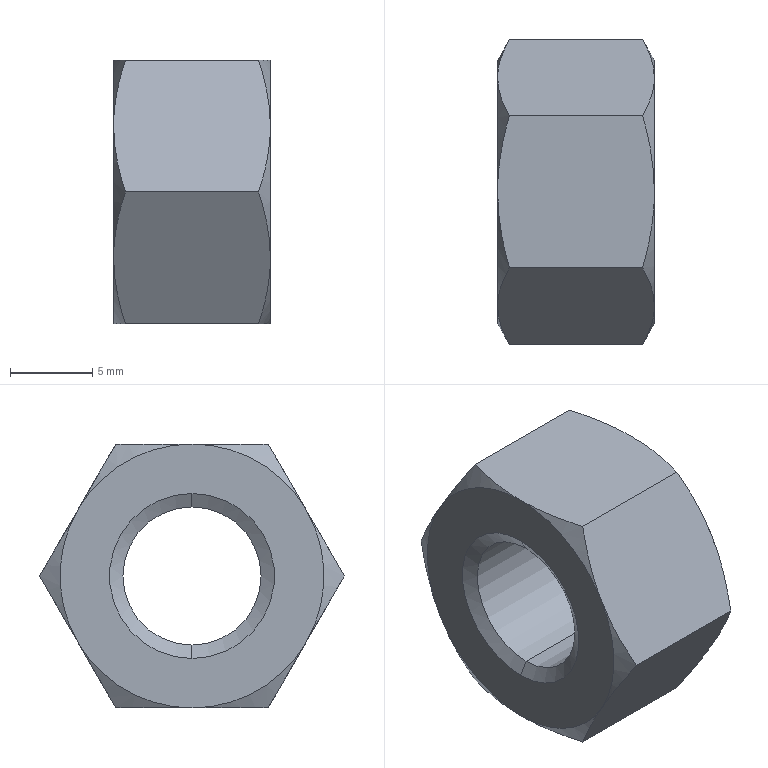Part | SolidWorks | features BaseBody 1 | 1 solid | 26 faces | box 9.5 x 18.475 x 16 mm | volume 1563 mm3 | cone 16 | plane 8 | cylinder 2 | commonest cylinder face diameters 8.376 x2
STEP:
#1=CARTESIAN_POINT('',(0.4688,0.,4.188));
#2=VERTEX_POINT('',#1);
#3=CARTESIAN_POINT('',(0.4688,0.,-4.188));
#4=VERTEX_POINT('',#3);
#5=CARTESIAN_POINT('',(0.4688,0.,0.));
#6=DIRECTION('',(1.,0.,0.));
#7=DIRECTION('',(0.,0.,-1.));
#8=AXIS2_PLACEMENT_3D('',#5,#6,#7);
#9=CIRCLE('',#8,4.188);
#10=EDGE_CURVE('',#2,#4,#9,.T.);
#11=ORIENTED_EDGE('',*,*,#10,.F.);
#12=CARTESIAN_POINT('',(9.031,0.,4.188));
#13=VERTEX_POINT('',#12);
#14=CARTESIAN_POINT('',(-16.722,0.,4.188));
#15=DIRECTION('',(1.,0.,0.));
#16=VECTOR('',#15,1000.);
#17=LINE('',#14,#16);
#18=EDGE_CURVE('',#2,#13,#17,.T.);
#19=ORIENTED_EDGE('',*,*,#18,.T.);
#20=CARTESIAN_POINT('',(9.031,0.,-4.188));
#21=VERTEX_POINT('',#20);
#22=CARTESIAN_POINT('',(9.031,0.,0.));
#23=DIRECTION('',(-1.,0.,0.));
#24=DIRECTION('',(0.,0.,-1.));
#25=AXIS2_PLACEMENT_3D('',#22,#23,#24);
#26=CIRCLE('',#25,4.188);
#27=EDGE_CURVE('',#21,#13,#26,.T.);
#28=ORIENTED_EDGE('',*,*,#27,.F.);
#29=CARTESIAN_POINT('',(-16.722,0.,-4.188));
#30=DIRECTION('',(1.,0.,0.));
#31=VECTOR('',#30,1000.);
#32=LINE('',#29,#31);
#33=EDGE_CURVE('',#4,#21,#32,.T.);
#34=ORIENTED_EDGE('',*,*,#33,.F.);
#35=EDGE_LOOP('',(#11,#19,#28,#34));
#36=FACE_OUTER_BOUND('',#35,.T.);
#37=CARTESIAN_POINT('',(-16.722,0.,0.));
#38=DIRECTION('',(1.,0.,0.));
#39=DIRECTION('',(0.,0.,-1.));
#40=AXIS2_PLACEMENT_3D('',#37,#38,#39);
#41=CYLINDRICAL_SURFACE('',#40,4.188);
#42=ADVANCED_FACE('',(#36),#41,.F.);
#43=ORIENTED_EDGE('',*,*,#10,.T.);
#44=CARTESIAN_POINT('',(0.,0.,-5.));
#45=VERTEX_POINT('',#44);
#46=CARTESIAN_POINT('',(0.,0.,-5.));
#47=DIRECTION('',(-0.5,0.,-0.866));
#48=VECTOR('',#47,1000.);
#49=LINE('',#46,#48);
#50=EDGE_CURVE('',#4,#45,#49,.T.);
#51=ORIENTED_EDGE('',*,*,#50,.T.);
#52=CARTESIAN_POINT('',(0.,0.,5.));
#53=VERTEX_POINT('',#52);
#54=CARTESIAN_POINT('',(0.,0.,0.));
#55=DIRECTION('',(1.,0.,0.));
#56=DIRECTION('',(0.,0.,1.));
#57=AXIS2_PLACEMENT_3D('',#54,#55,#56);
#58=CIRCLE('',#57,5.);
#59=EDGE_CURVE('',#53,#45,#58,.T.);
#60=ORIENTED_EDGE('',*,*,#59,.F.);
#61=CARTESIAN_POINT('',(0.,0.,5.));
#62=DIRECTION('',(-0.5,0.,0.866));
#63=VECTOR('',#62,1000.);
#64=LINE('',#61,#63);
#65=EDGE_CURVE('',#2,#53,#64,.T.);
#66=ORIENTED_EDGE('',*,*,#65,.F.);
#67=EDGE_LOOP('',(#43,#51,#60,#66));
#68=FACE_OUTER_BOUND('',#67,.T.);
#69=CARTESIAN_POINT('',(0.,0.,0.));
#70=DIRECTION('',(-1.,0.,0.));
#71=DIRECTION('',(0.,0.,1.));
#72=AXIS2_PLACEMENT_3D('',#69,#70,#71);
#73=CONICAL_SURFACE('',#72,5.,1.047);
#74=ADVANCED_FACE('',(#68),#73,.F.);
#75=ORIENTED_EDGE('',*,*,#27,.T.);
#76=CARTESIAN_POINT('',(9.5,0.,5.));
#77=VERTEX_POINT('',#76);
#78=CARTESIAN_POINT('',(9.5,0.,5.));
#79=DIRECTION('',(0.5,0.,0.866));
#80=VECTOR('',#79,1000.);
#81=LINE('',#78,#80);
#82=EDGE_CURVE('',#13,#77,#81,.T.);
#83=ORIENTED_EDGE('',*,*,#82,.T.);
#84=CARTESIAN_POINT('',(9.5,0.,-5.));
#85=VERTEX_POINT('',#84);
#86=CARTESIAN_POINT('',(9.5,0.,0.));
#87=DIRECTION('',(-1.,0.,0.));
#88=DIRECTION('',(0.,0.,-1.));
#89=AXIS2_PLACEMENT_3D('',#86,#87,#88);
#90=CIRCLE('',#89,5.);
#91=EDGE_CURVE('',#85,#77,#90,.T.);
#92=ORIENTED_EDGE('',*,*,#91,.F.);
#93=CARTESIAN_POINT('',(9.5,0.,-5.));
#94=DIRECTION('',(0.5,0.,-0.866));
#95=VECTOR('',#94,1000.);
#96=LINE('',#93,#95);
#97=EDGE_CURVE('',#21,#85,#96,.T.);
#98=ORIENTED_EDGE('',*,*,#97,.F.);
#99=EDGE_LOOP('',(#75,#83,#92,#98));
#100=FACE_OUTER_BOUND('',#99,.T.);
#101=CARTESIAN_POINT('',(9.5,0.,0.));
#102=DIRECTION('',(1.,0.,0.));
#103=DIRECTION('',(0.,0.,-1.));
#104=AXIS2_PLACEMENT_3D('',#101,#102,#103);
#105=CONICAL_SURFACE('',#104,5.,1.047);
#106=ADVANCED_FACE('',(#100),#105,.F.);
#107=ORIENTED_EDGE('',*,*,#18,.F.);
#108=CARTESIAN_POINT('',(0.4688,0.,0.));
#109=DIRECTION('',(1.,0.,0.));
#110=DIRECTION('',(0.,0.,-1.));
#111=AXIS2_PLACEMENT_3D('',#108,#109,#110);
#112=CIRCLE('',#111,4.188);
#113=EDGE_CURVE('',#4,#2,#112,.T.);
#114=ORIENTED_EDGE('',*,*,#113,.F.);
#115=ORIENTED_EDGE('',*,*,#33,.T.);
#116=CARTESIAN_POINT('',(9.031,0.,0.));
#117=DIRECTION('',(-1.,0.,0.));
#118=DIRECTION('',(0.,0.,-1.));
#119=AXIS2_PLACEMENT_3D('',#116,#117,#118);
#120=CIRCLE('',#119,4.188);
#121=EDGE_CURVE('',#13,#21,#120,.T.);
#122=ORIENTED_EDGE('',*,*,#121,.F.);
#123=EDGE_LOOP('',(#107,#114,#115,#122));
#124=FACE_OUTER_BOUND('',#123,.T.);
#125=CARTESIAN_POINT('',(-16.722,0.,0.));
#126=DIRECTION('',(1.,0.,0.));
#127=DIRECTION('',(0.,0.,-1.));
#128=AXIS2_PLACEMENT_3D('',#125,#126,#127);
#129=CYLINDRICAL_SURFACE('',#128,4.188);
#130=ADVANCED_FACE('',(#124),#129,.F.);
#131=ORIENTED_EDGE('',*,*,#50,.F.);
#132=ORIENTED_EDGE('',*,*,#113,.T.);
#133=ORIENTED_EDGE('',*,*,#65,.T.);
#134=CARTESIAN_POINT('',(0.,0.,0.));
#135=DIRECTION('',(1.,0.,0.));
#136=DIRECTION('',(0.,0.,1.));
#137=AXIS2_PLACEMENT_3D('',#134,#135,#136);
#138=CIRCLE('',#137,5.);
#139=EDGE_CURVE('',#45,#53,#138,.T.);
#140=ORIENTED_EDGE('',*,*,#139,.F.);
#141=EDGE_LOOP('',(#131,#132,#133,#140));
#142=FACE_OUTER_BOUND('',#141,.T.);
#143=CARTESIAN_POINT('',(0.,0.,0.));
#144=DIRECTION('',(-1.,0.,0.));
#145=DIRECTION('',(0.,0.,1.));
#146=AXIS2_PLACEMENT_3D('',#143,#144,#145);
#147=CONICAL_SURFACE('',#146,5.,1.047);
#148=ADVANCED_FACE('',(#142),#147,.F.);
#149=ORIENTED_EDGE('',*,*,#82,.F.);
#150=ORIENTED_EDGE('',*,*,#121,.T.);
#151=ORIENTED_EDGE('',*,*,#97,.T.);
#152=CARTESIAN_POINT('',(9.5,0.,0.));
#153=DIRECTION('',(-1.,0.,0.));
#154=DIRECTION('',(0.,0.,-1.));
#155=AXIS2_PLACEMENT_3D('',#152,#153,#154);
#156=CIRCLE('',#155,5.);
#157=EDGE_CURVE('',#77,#85,#156,.T.);
#158=ORIENTED_EDGE('',*,*,#157,.F.);
#159=EDGE_LOOP('',(#149,#150,#151,#158));
#160=FACE_OUTER_BOUND('',#159,.T.);
#161=CARTESIAN_POINT('',(9.5,0.,0.));
#162=DIRECTION('',(1.,0.,0.));
#163=DIRECTION('',(0.,0.,-1.));
#164=AXIS2_PLACEMENT_3D('',#161,#162,#163);
#165=CONICAL_SURFACE('',#164,5.,1.047);
#166=ADVANCED_FACE('',(#160),#165,.F.);
#167=ORIENTED_EDGE('',*,*,#59,.T.);
#168=ORIENTED_EDGE('',*,*,#139,.T.);
#169=EDGE_LOOP('',(#167,#168));
#170=FACE_BOUND('',#169,.T.);
#171=CARTESIAN_POINT('',(0.,0.,8.));
#172=VERTEX_POINT('',#171);
#173=CARTESIAN_POINT('',(0.,-6.928,4.));
#174=VERTEX_POINT('',#173);
#175=CARTESIAN_POINT('',(0.,0.,0.));
#176=DIRECTION('',(1.,0.,0.));
#177=DIRECTION('',(0.,0.,-1.));
#178=AXIS2_PLACEMENT_3D('',#175,#176,#177);
#179=CIRCLE('',#178,8.);
#180=EDGE_CURVE('',#172,#174,#179,.T.);
#181=ORIENTED_EDGE('',*,*,#180,.F.);
#182=CARTESIAN_POINT('',(0.,6.928,4.));
#183=VERTEX_POINT('',#182);
#184=CARTESIAN_POINT('',(0.,0.,0.));
#185=DIRECTION('',(1.,0.,0.));
#186=DIRECTION('',(0.,0.,-1.));
#187=AXIS2_PLACEMENT_3D('',#184,#185,#186);
#188=CIRCLE('',#187,8.);
#189=EDGE_CURVE('',#183,#172,#188,.T.);
#190=ORIENTED_EDGE('',*,*,#189,.F.);
#191=CARTESIAN_POINT('',(0.,6.928,-4.));
#192=VERTEX_POINT('',#191);
#193=CARTESIAN_POINT('',(0.,0.,0.));
#194=DIRECTION('',(1.,0.,0.));
#195=DIRECTION('',(0.,0.,-1.));
#196=AXIS2_PLACEMENT_3D('',#193,#194,#195);
#197=CIRCLE('',#196,8.);
#198=EDGE_CURVE('',#192,#183,#197,.T.);
#199=ORIENTED_EDGE('',*,*,#198,.F.);
#200=CARTESIAN_POINT('',(0.,0.,-8.));
#201=VERTEX_POINT('',#200);
#202=CARTESIAN_POINT('',(0.,0.,0.));
#203=DIRECTION('',(1.,0.,0.));
#204=DIRECTION('',(0.,0.,-1.));
#205=AXIS2_PLACEMENT_3D('',#202,#203,#204);
#206=CIRCLE('',#205,8.);
#207=EDGE_CURVE('',#201,#192,#206,.T.);
#208=ORIENTED_EDGE('',*,*,#207,.F.);
#209=CARTESIAN_POINT('',(0.,-6.928,-4.));
#210=VERTEX_POINT('',#209);
#211=CARTESIAN_POINT('',(0.,0.,0.));
#212=DIRECTION('',(1.,0.,0.));
#213=DIRECTION('',(0.,0.,-1.));
#214=AXIS2_PLACEMENT_3D('',#211,#212,#213);
#215=CIRCLE('',#214,8.);
#216=EDGE_CURVE('',#210,#201,#215,.T.);
#217=ORIENTED_EDGE('',*,*,#216,.F.);
#218=CARTESIAN_POINT('',(0.,0.,0.));
#219=DIRECTION('',(1.,0.,0.));
#220=DIRECTION('',(0.,0.,-1.));
#221=AXIS2_PLACEMENT_3D('',#218,#219,#220);
#222=CIRCLE('',#221,8.);
#223=EDGE_CURVE('',#174,#210,#222,.T.);
#224=ORIENTED_EDGE('',*,*,#223,.F.);
#225=EDGE_LOOP('',(#181,#190,#199,#208,#217,#224));
#226=FACE_OUTER_BOUND('',#225,.T.);
#227=CARTESIAN_POINT('',(0.,0.,0.));
#228=DIRECTION('',(1.,0.,0.));
#229=DIRECTION('',(0.,0.,-1.));
#230=AXIS2_PLACEMENT_3D('',#227,#228,#229);
#231=PLANE('',#230);
#232=ADVANCED_FACE('',(#170,#226),#231,.F.);
#233=ORIENTED_EDGE('',*,*,#91,.T.);
#234=ORIENTED_EDGE('',*,*,#157,.T.);
#235=EDGE_LOOP('',(#233,#234));
#236=FACE_BOUND('',#235,.T.);
#237=CARTESIAN_POINT('',(9.5,0.,8.));
#238=VERTEX_POINT('',#237);
#239=CARTESIAN_POINT('',(9.5,-6.928,4.));
#240=VERTEX_POINT('',#239);
#241=CARTESIAN_POINT('',(9.5,0.,0.));
#242=DIRECTION('',(1.,0.,0.));
#243=DIRECTION('',(0.,0.,1.));
#244=AXIS2_PLACEMENT_3D('',#241,#242,#243);
#245=CIRCLE('',#244,8.);
#246=EDGE_CURVE('',#238,#240,#245,.T.);
#247=ORIENTED_EDGE('',*,*,#246,.T.);
#248=CARTESIAN_POINT('',(9.5,-6.928,-4.));
#249=VERTEX_POINT('',#248);
#250=CARTESIAN_POINT('',(9.5,0.,0.));
#251=DIRECTION('',(1.,0.,0.));
#252=DIRECTION('',(0.,0.,1.));
#253=AXIS2_PLACEMENT_3D('',#250,#251,#252);
#254=CIRCLE('',#253,8.);
#255=EDGE_CURVE('',#240,#249,#254,.T.);
#256=ORIENTED_EDGE('',*,*,#255,.T.);
#257=CARTESIAN_POINT('',(9.5,0.,-8.));
#258=VERTEX_POINT('',#257);
#259=CARTESIAN_POINT('',(9.5,0.,0.));
#260=DIRECTION('',(1.,0.,0.));
#261=DIRECTION('',(0.,0.,1.));
#262=AXIS2_PLACEMENT_3D('',#259,#260,#261);
#263=CIRCLE('',#262,8.);
#264=EDGE_CURVE('',#249,#258,#263,.T.);
#265=ORIENTED_EDGE('',*,*,#264,.T.);
#266=CARTESIAN_POINT('',(9.5,6.928,-4.));
#267=VERTEX_POINT('',#266);
#268=CARTESIAN_POINT('',(9.5,0.,0.));
#269=DIRECTION('',(1.,0.,0.));
#270=DIRECTION('',(0.,0.,1.));
#271=AXIS2_PLACEMENT_3D('',#268,#269,#270);
#272=CIRCLE('',#271,8.);
#273=EDGE_CURVE('',#258,#267,#272,.T.);
#274=ORIENTED_EDGE('',*,*,#273,.T.);
#275=CARTESIAN_POINT('',(9.5,6.928,4.));
#276=VERTEX_POINT('',#275);
#277=CARTESIAN_POINT('',(9.5,0.,0.));
#278=DIRECTION('',(1.,0.,0.));
#279=DIRECTION('',(0.,0.,1.));
#280=AXIS2_PLACEMENT_3D('',#277,#278,#279);
#281=CIRCLE('',#280,8.);
#282=EDGE_CURVE('',#267,#276,#281,.T.);
#283=ORIENTED_EDGE('',*,*,#282,.T.);
#284=CARTESIAN_POINT('',(9.5,0.,0.));
#285=DIRECTION('',(1.,0.,0.));
#286=DIRECTION('',(0.,0.,1.));
#287=AXIS2_PLACEMENT_3D('',#284,#285,#286);
#288=CIRCLE('',#287,8.);
#289=EDGE_CURVE('',#276,#238,#288,.T.);
#290=ORIENTED_EDGE('',*,*,#289,.T.);
#291=EDGE_LOOP('',(#247,#256,#265,#274,#283,#290));
#292=FACE_OUTER_BOUND('',#291,.T.);
#293=CARTESIAN_POINT('',(9.5,0.,0.));
#294=DIRECTION('',(1.,0.,0.));
#295=DIRECTION('',(0.,0.,-1.));
#296=AXIS2_PLACEMENT_3D('',#293,#294,#295);
#297=PLANE('',#296);
#298=ADVANCED_FACE('',(#236,#292),#297,.T.);
#299=ORIENTED_EDGE('',*,*,#223,.T.);
#300=CARTESIAN_POINT('',(0.7145,-9.238,0.000000014));
#301=VERTEX_POINT('',#300);
#302=CARTESIAN_POINT('',(0.,-6.928,-4.));
#303=CARTESIAN_POINT('',(0.,-7.322,-3.317));
#304=CARTESIAN_POINT('',(0.06831,-7.711,-2.644));
#305=CARTESIAN_POINT('',(0.3171,-8.48,-1.312));
#306=CARTESIAN_POINT('',(0.4967,-8.86,-0.6534));
#307=CARTESIAN_POINT('',(0.7145,-9.238,0.000000014));
#308=B_SPLINE_CURVE_WITH_KNOTS('',3,(#302,#303,#304,#305,#306,#307),.UNSPECIFIED.,.F.,.F.,(4,2,4),(0.,0.002337,0.004674),.UNSPECIFIED.);
#309=EDGE_CURVE('',#210,#301,#308,.T.);
#310=ORIENTED_EDGE('',*,*,#309,.T.);
#311=CARTESIAN_POINT('',(0.7145,-9.238,0.000000014));
#312=CARTESIAN_POINT('',(0.4967,-8.86,0.6534));
#313=CARTESIAN_POINT('',(0.3171,-8.48,1.312));
#314=CARTESIAN_POINT('',(0.06831,-7.711,2.644));
#315=CARTESIAN_POINT('',(0.,-7.322,3.317));
#316=CARTESIAN_POINT('',(0.,-6.928,4.));
#317=B_SPLINE_CURVE_WITH_KNOTS('',3,(#311,#312,#313,#314,#315,#316),.UNSPECIFIED.,.F.,.F.,(4,2,4),(0.,0.002337,0.004674),.UNSPECIFIED.);
#318=EDGE_CURVE('',#301,#174,#317,.T.);
#319=ORIENTED_EDGE('',*,*,#318,.T.);
#320=EDGE_LOOP('',(#299,#310,#319));
#321=FACE_OUTER_BOUND('',#320,.T.);
#322=CARTESIAN_POINT('',(0.7188,0.,0.));
#323=DIRECTION('',(1.,0.,0.));
#324=DIRECTION('',(0.,0.,-1.));
#325=AXIS2_PLACEMENT_3D('',#322,#323,#324);
#326=CONICAL_SURFACE('',#325,9.245,1.047);
#327=ADVANCED_FACE('',(#321),#326,.T.);
#328=ORIENTED_EDGE('',*,*,#180,.T.);
#329=CARTESIAN_POINT('',(0.7145,-4.619,8.));
#330=VERTEX_POINT('',#329);
#331=CARTESIAN_POINT('',(0.,-6.928,4.));
#332=CARTESIAN_POINT('',(0.,-6.534,4.683));
#333=CARTESIAN_POINT('',(0.06831,-6.145,5.356));
#334=CARTESIAN_POINT('',(0.3171,-5.376,6.688));
#335=CARTESIAN_POINT('',(0.4967,-4.996,7.347));
#336=CARTESIAN_POINT('',(0.7145,-4.619,8.));
#337=B_SPLINE_CURVE_WITH_KNOTS('',3,(#331,#332,#333,#334,#335,#336),.UNSPECIFIED.,.F.,.F.,(4,2,4),(0.,0.002337,0.004674),.UNSPECIFIED.);
#338=EDGE_CURVE('',#174,#330,#337,.T.);
#339=ORIENTED_EDGE('',*,*,#338,.T.);
#340=CARTESIAN_POINT('',(0.7145,-4.619,8.));
#341=CARTESIAN_POINT('',(0.4967,-3.864,8.));
#342=CARTESIAN_POINT('',(0.3171,-3.104,8.));
#343=CARTESIAN_POINT('',(0.06831,-1.566,8.));
#344=CARTESIAN_POINT('',(0.,-0.7882,8.));
#345=CARTESIAN_POINT('',(0.,0.,8.));
#346=B_SPLINE_CURVE_WITH_KNOTS('',3,(#340,#341,#342,#343,#344,#345),.UNSPECIFIED.,.F.,.F.,(4,2,4),(0.,0.002337,0.004674),.UNSPECIFIED.);
#347=EDGE_CURVE('',#330,#172,#346,.T.);
#348=ORIENTED_EDGE('',*,*,#347,.T.);
#349=EDGE_LOOP('',(#328,#339,#348));
#350=FACE_OUTER_BOUND('',#349,.T.);
#351=CARTESIAN_POINT('',(0.7188,0.,0.));
#352=DIRECTION('',(1.,0.,0.));
#353=DIRECTION('',(0.,0.,-1.));
#354=AXIS2_PLACEMENT_3D('',#351,#352,#353);
#355=CONICAL_SURFACE('',#354,9.245,1.047);
#356=ADVANCED_FACE('',(#350),#355,.T.);
#357=ORIENTED_EDGE('',*,*,#189,.T.);
#358=CARTESIAN_POINT('',(0.7145,4.619,8.));
#359=VERTEX_POINT('',#358);
#360=CARTESIAN_POINT('',(0.,0.,8.));
#361=CARTESIAN_POINT('',(0.,0.7882,8.));
#362=CARTESIAN_POINT('',(0.06831,1.566,8.));
#363=CARTESIAN_POINT('',(0.3171,3.104,8.));
#364=CARTESIAN_POINT('',(0.4967,3.864,8.));
#365=CARTESIAN_POINT('',(0.7145,4.619,8.));
#366=B_SPLINE_CURVE_WITH_KNOTS('',3,(#360,#361,#362,#363,#364,#365),.UNSPECIFIED.,.F.,.F.,(4,2,4),(0.,0.002337,0.004674),.UNSPECIFIED.);
#367=EDGE_CURVE('',#172,#359,#366,.T.);
#368=ORIENTED_EDGE('',*,*,#367,.T.);
#369=CARTESIAN_POINT('',(0.7145,4.619,8.));
#370=CARTESIAN_POINT('',(0.4967,4.996,7.347));
#371=CARTESIAN_POINT('',(0.3171,5.376,6.688));
#372=CARTESIAN_POINT('',(0.06831,6.145,5.356));
#373=CARTESIAN_POINT('',(0.,6.534,4.683));
#374=CARTESIAN_POINT('',(0.,6.928,4.));
#375=B_SPLINE_CURVE_WITH_KNOTS('',3,(#369,#370,#371,#372,#373,#374),.UNSPECIFIED.,.F.,.F.,(4,2,4),(0.,0.002337,0.004674),.UNSPECIFIED.);
#376=EDGE_CURVE('',#359,#183,#375,.T.);
#377=ORIENTED_EDGE('',*,*,#376,.T.);
#378=EDGE_LOOP('',(#357,#368,#377));
#379=FACE_OUTER_BOUND('',#378,.T.);
#380=CARTESIAN_POINT('',(0.7188,0.,0.));
#381=DIRECTION('',(1.,0.,0.));
#382=DIRECTION('',(0.,0.,-1.));
#383=AXIS2_PLACEMENT_3D('',#380,#381,#382);
#384=CONICAL_SURFACE('',#383,9.245,1.047);
#385=ADVANCED_FACE('',(#379),#384,.T.);
#386=ORIENTED_EDGE('',*,*,#198,.T.);
#387=CARTESIAN_POINT('',(0.7145,9.238,-0.000000014));
#388=VERTEX_POINT('',#387);
#389=CARTESIAN_POINT('',(0.,6.928,4.));
#390=CARTESIAN_POINT('',(0.,7.322,3.317));
#391=CARTESIAN_POINT('',(0.06831,7.711,2.644));
#392=CARTESIAN_POINT('',(0.3171,8.48,1.312));
#393=CARTESIAN_POINT('',(0.4967,8.86,0.6534));
#394=CARTESIAN_POINT('',(0.7145,9.238,-0.000000014));
#395=B_SPLINE_CURVE_WITH_KNOTS('',3,(#389,#390,#391,#392,#393,#394),.UNSPECIFIED.,.F.,.F.,(4,2,4),(0.,0.002337,0.004674),.UNSPECIFIED.);
#396=EDGE_CURVE('',#183,#388,#395,.T.);
#397=ORIENTED_EDGE('',*,*,#396,.T.);
#398=CARTESIAN_POINT('',(0.7145,9.238,-0.000000014));
#399=CARTESIAN_POINT('',(0.4967,8.86,-0.6534));
#400=CARTESIAN_POINT('',(0.3171,8.48,-1.312));
#401=CARTESIAN_POINT('',(0.06831,7.711,-2.644));
#402=CARTESIAN_POINT('',(0.,7.322,-3.317));
#403=CARTESIAN_POINT('',(0.,6.928,-4.));
#404=B_SPLINE_CURVE_WITH_KNOTS('',3,(#398,#399,#400,#401,#402,#403),.UNSPECIFIED.,.F.,.F.,(4,2,4),(0.,0.002337,0.004674),.UNSPECIFIED.);
#405=EDGE_CURVE('',#388,#192,#404,.T.);
#406=ORIENTED_EDGE('',*,*,#405,.T.);
#407=EDGE_LOOP('',(#386,#397,#406));
#408=FACE_OUTER_BOUND('',#407,.T.);
#409=CARTESIAN_POINT('',(0.7188,0.,0.));
#410=DIRECTION('',(1.,0.,0.));
#411=DIRECTION('',(0.,0.,-1.));
#412=AXIS2_PLACEMENT_3D('',#409,#410,#411);
#413=CONICAL_SURFACE('',#412,9.245,1.047);
#414=ADVANCED_FACE('',(#408),#413,.T.);
#415=CARTESIAN_POINT('',(0.7145,4.619,-8.));
#416=VERTEX_POINT('',#415);
#417=CARTESIAN_POINT('',(0.7145,4.619,-8.));
#418=CARTESIAN_POINT('',(0.4967,3.864,-8.));
#419=CARTESIAN_POINT('',(0.3171,3.104,-8.));
#420=CARTESIAN_POINT('',(0.06831,1.566,-8.));
#421=CARTESIAN_POINT('',(0.,0.7882,-8.));
#422=CARTESIAN_POINT('',(0.,0.,-8.));
#423=B_SPLINE_CURVE_WITH_KNOTS('',3,(#417,#418,#419,#420,#421,#422),.UNSPECIFIED.,.F.,.F.,(4,2,4),(0.,0.002337,0.004674),.UNSPECIFIED.);
#424=EDGE_CURVE('',#416,#201,#423,.T.);
#425=ORIENTED_EDGE('',*,*,#424,.T.);
#426=ORIENTED_EDGE('',*,*,#207,.T.);
#427=CARTESIAN_POINT('',(0.,6.928,-4.));
#428=CARTESIAN_POINT('',(0.,6.534,-4.683));
#429=CARTESIAN_POINT('',(0.06831,6.145,-5.356));
#430=CARTESIAN_POINT('',(0.3171,5.376,-6.688));
#431=CARTESIAN_POINT('',(0.4967,4.996,-7.347));
#432=CARTESIAN_POINT('',(0.7145,4.619,-8.));
#433=B_SPLINE_CURVE_WITH_KNOTS('',3,(#427,#428,#429,#430,#431,#432),.UNSPECIFIED.,.F.,.F.,(4,2,4),(0.,0.002337,0.004674),.UNSPECIFIED.);
#434=EDGE_CURVE('',#192,#416,#433,.T.);
#435=ORIENTED_EDGE('',*,*,#434,.T.);
#436=EDGE_LOOP('',(#425,#426,#435));
#437=FACE_OUTER_BOUND('',#436,.T.);
#438=CARTESIAN_POINT('',(0.7188,0.,0.));
#439=DIRECTION('',(1.,0.,0.));
#440=DIRECTION('',(0.,0.,-1.));
#441=AXIS2_PLACEMENT_3D('',#438,#439,#440);
#442=CONICAL_SURFACE('',#441,9.245,1.047);
#443=ADVANCED_FACE('',(#437),#442,.T.);
#444=CARTESIAN_POINT('',(0.7145,-4.619,-8.));
#445=VERTEX_POINT('',#444);
#446=CARTESIAN_POINT('',(0.7145,-4.619,-8.));
#447=CARTESIAN_POINT('',(0.4967,-4.996,-7.347));
#448=CARTESIAN_POINT('',(0.3171,-5.376,-6.688));
#449=CARTESIAN_POINT('',(0.06831,-6.145,-5.356));
#450=CARTESIAN_POINT('',(0.,-6.534,-4.683));
#451=CARTESIAN_POINT('',(0.,-6.928,-4.));
#452=B_SPLINE_CURVE_WITH_KNOTS('',3,(#446,#447,#448,#449,#450,#451),.UNSPECIFIED.,.F.,.F.,(4,2,4),(0.,0.002337,0.004674),.UNSPECIFIED.);
#453=EDGE_CURVE('',#445,#210,#452,.T.);
#454=ORIENTED_EDGE('',*,*,#453,.T.);
#455=ORIENTED_EDGE('',*,*,#216,.T.);
#456=CARTESIAN_POINT('',(0.,0.,-8.));
#457=CARTESIAN_POINT('',(0.,-0.7882,-8.));
#458=CARTESIAN_POINT('',(0.06831,-1.566,-8.));
#459=CARTESIAN_POINT('',(0.3171,-3.104,-8.));
#460=CARTESIAN_POINT('',(0.4967,-3.864,-8.));
#461=CARTESIAN_POINT('',(0.7145,-4.619,-8.));
#462=B_SPLINE_CURVE_WITH_KNOTS('',3,(#456,#457,#458,#459,#460,#461),.UNSPECIFIED.,.F.,.F.,(4,2,4),(0.,0.002337,0.004674),.UNSPECIFIED.);
#463=EDGE_CURVE('',#201,#445,#462,.T.);
#464=ORIENTED_EDGE('',*,*,#463,.T.);
#465=EDGE_LOOP('',(#454,#455,#464));
#466=FACE_OUTER_BOUND('',#465,.T.);
#467=CARTESIAN_POINT('',(0.7188,0.,0.));
#468=DIRECTION('',(1.,0.,0.));
#469=DIRECTION('',(0.,0.,-1.));
#470=AXIS2_PLACEMENT_3D('',#467,#468,#469);
#471=CONICAL_SURFACE('',#470,9.245,1.047);
#472=ADVANCED_FACE('',(#466),#471,.T.);
#473=CARTESIAN_POINT('',(8.785,-9.238,0.000000038));
#474=VERTEX_POINT('',#473);
#475=CARTESIAN_POINT('',(8.785,-9.238,0.000000038));
#476=CARTESIAN_POINT('',(9.003,-8.86,-0.6534));
#477=CARTESIAN_POINT('',(9.183,-8.48,-1.312));
#478=CARTESIAN_POINT('',(9.432,-7.711,-2.644));
#479=CARTESIAN_POINT('',(9.5,-7.322,-3.317));
#480=CARTESIAN_POINT('',(9.5,-6.928,-4.));
#481=B_SPLINE_CURVE_WITH_KNOTS('',3,(#475,#476,#477,#478,#479,#480),.UNSPECIFIED.,.F.,.F.,(4,2,4),(0.,0.002337,0.004674),.UNSPECIFIED.);
#482=EDGE_CURVE('',#474,#249,#481,.T.);
#483=ORIENTED_EDGE('',*,*,#482,.T.);
#484=ORIENTED_EDGE('',*,*,#255,.F.);
#485=CARTESIAN_POINT('',(9.5,-6.928,4.));
#486=CARTESIAN_POINT('',(9.5,-7.322,3.317));
#487=CARTESIAN_POINT('',(9.432,-7.711,2.644));
#488=CARTESIAN_POINT('',(9.183,-8.48,1.312));
#489=CARTESIAN_POINT('',(9.003,-8.86,0.6534));
#490=CARTESIAN_POINT('',(8.785,-9.238,0.000000038));
#491=B_SPLINE_CURVE_WITH_KNOTS('',3,(#485,#486,#487,#488,#489,#490),.UNSPECIFIED.,.F.,.F.,(4,2,4),(0.,0.002337,0.004674),.UNSPECIFIED.);
#492=EDGE_CURVE('',#240,#474,#491,.T.);
#493=ORIENTED_EDGE('',*,*,#492,.T.);
#494=EDGE_LOOP('',(#483,#484,#493));
#495=FACE_OUTER_BOUND('',#494,.T.);
#496=CARTESIAN_POINT('',(8.781,0.,0.));
#497=DIRECTION('',(-1.,0.,0.));
#498=DIRECTION('',(0.,0.,1.));
#499=AXIS2_PLACEMENT_3D('',#496,#497,#498);
#500=CONICAL_SURFACE('',#499,9.245,1.047);
#501=ADVANCED_FACE('',(#495),#500,.T.);
#502=CARTESIAN_POINT('',(8.785,-4.619,8.));
#503=VERTEX_POINT('',#502);
#504=CARTESIAN_POINT('',(8.785,-4.619,8.));
#505=CARTESIAN_POINT('',(9.003,-4.996,7.347));
#506=CARTESIAN_POINT('',(9.183,-5.376,6.688));
#507=CARTESIAN_POINT('',(9.432,-6.145,5.356));
#508=CARTESIAN_POINT('',(9.5,-6.534,4.683));
#509=CARTESIAN_POINT('',(9.5,-6.928,4.));
#510=B_SPLINE_CURVE_WITH_KNOTS('',3,(#504,#505,#506,#507,#508,#509),.UNSPECIFIED.,.F.,.F.,(4,2,4),(0.,0.002337,0.004674),.UNSPECIFIED.);
#511=EDGE_CURVE('',#503,#240,#510,.T.);
#512=ORIENTED_EDGE('',*,*,#511,.T.);
#513=ORIENTED_EDGE('',*,*,#246,.F.);
#514=CARTESIAN_POINT('',(9.5,0.,8.));
#515=CARTESIAN_POINT('',(9.5,-0.7882,8.));
#516=CARTESIAN_POINT('',(9.432,-1.566,8.));
#517=CARTESIAN_POINT('',(9.183,-3.104,8.));
#518=CARTESIAN_POINT('',(9.003,-3.864,8.));
#519=CARTESIAN_POINT('',(8.785,-4.619,8.));
#520=B_SPLINE_CURVE_WITH_KNOTS('',3,(#514,#515,#516,#517,#518,#519),.UNSPECIFIED.,.F.,.F.,(4,2,4),(0.,0.002337,0.004674),.UNSPECIFIED.);
#521=EDGE_CURVE('',#238,#503,#520,.T.);
#522=ORIENTED_EDGE('',*,*,#521,.T.);
#523=EDGE_LOOP('',(#512,#513,#522));
#524=FACE_OUTER_BOUND('',#523,.T.);
#525=CARTESIAN_POINT('',(8.781,0.,0.));
#526=DIRECTION('',(-1.,0.,0.));
#527=DIRECTION('',(0.,0.,1.));
#528=AXIS2_PLACEMENT_3D('',#525,#526,#527);
#529=CONICAL_SURFACE('',#528,9.245,1.047);
#530=ADVANCED_FACE('',(#524),#529,.T.);
#531=CARTESIAN_POINT('',(8.785,4.619,8.));
#532=VERTEX_POINT('',#531);
#533=CARTESIAN_POINT('',(8.785,4.619,8.));
#534=CARTESIAN_POINT('',(9.003,3.864,8.));
#535=CARTESIAN_POINT('',(9.183,3.104,8.));
#536=CARTESIAN_POINT('',(9.432,1.566,8.));
#537=CARTESIAN_POINT('',(9.5,0.7882,8.));
#538=CARTESIAN_POINT('',(9.5,0.,8.));
#539=B_SPLINE_CURVE_WITH_KNOTS('',3,(#533,#534,#535,#536,#537,#538),.UNSPECIFIED.,.F.,.F.,(4,2,4),(0.,0.002337,0.004674),.UNSPECIFIED.);
#540=EDGE_CURVE('',#532,#238,#539,.T.);
#541=ORIENTED_EDGE('',*,*,#540,.T.);
#542=ORIENTED_EDGE('',*,*,#289,.F.);
#543=CARTESIAN_POINT('',(9.5,6.928,4.));
#544=CARTESIAN_POINT('',(9.5,6.534,4.683));
#545=CARTESIAN_POINT('',(9.432,6.145,5.356));
#546=CARTESIAN_POINT('',(9.183,5.376,6.688));
#547=CARTESIAN_POINT('',(9.003,4.996,7.347));
#548=CARTESIAN_POINT('',(8.785,4.619,8.));
#549=B_SPLINE_CURVE_WITH_KNOTS('',3,(#543,#544,#545,#546,#547,#548),.UNSPECIFIED.,.F.,.F.,(4,2,4),(0.,0.002337,0.004674),.UNSPECIFIED.);
#550=EDGE_CURVE('',#276,#532,#549,.T.);
#551=ORIENTED_EDGE('',*,*,#550,.T.);
#552=EDGE_LOOP('',(#541,#542,#551));
#553=FACE_OUTER_BOUND('',#552,.T.);
#554=CARTESIAN_POINT('',(8.781,0.,0.));
#555=DIRECTION('',(-1.,0.,0.));
#556=DIRECTION('',(0.,0.,1.));
#557=AXIS2_PLACEMENT_3D('',#554,#555,#556);
#558=CONICAL_SURFACE('',#557,9.245,1.047);
#559=ADVANCED_FACE('',(#553),#558,.T.);
#560=ORIENTED_EDGE('',*,*,#282,.F.);
#561=CARTESIAN_POINT('',(8.785,9.238,0.000000014));
#562=VERTEX_POINT('',#561);
#563=CARTESIAN_POINT('',(9.5,6.928,-4.));
#564=CARTESIAN_POINT('',(9.5,7.322,-3.317));
#565=CARTESIAN_POINT('',(9.432,7.711,-2.644));
#566=CARTESIAN_POINT('',(9.183,8.48,-1.312));
#567=CARTESIAN_POINT('',(9.003,8.86,-0.6534));
#568=CARTESIAN_POINT('',(8.785,9.238,0.000000014));
#569=B_SPLINE_CURVE_WITH_KNOTS('',3,(#563,#564,#565,#566,#567,#568),.UNSPECIFIED.,.F.,.F.,(4,2,4),(0.,0.002337,0.004674),.UNSPECIFIED.);
#570=EDGE_CURVE('',#267,#562,#569,.T.);
#571=ORIENTED_EDGE('',*,*,#570,.T.);
#572=CARTESIAN_POINT('',(8.785,9.238,0.000000014));
#573=CARTESIAN_POINT('',(9.003,8.86,0.6534));
#574=CARTESIAN_POINT('',(9.183,8.48,1.312));
#575=CARTESIAN_POINT('',(9.432,7.711,2.644));
#576=CARTESIAN_POINT('',(9.5,7.322,3.317));
#577=CARTESIAN_POINT('',(9.5,6.928,4.));
#578=B_SPLINE_CURVE_WITH_KNOTS('',3,(#572,#573,#574,#575,#576,#577),.UNSPECIFIED.,.F.,.F.,(4,2,4),(0.,0.002337,0.004674),.UNSPECIFIED.);
#579=EDGE_CURVE('',#562,#276,#578,.T.);
#580=ORIENTED_EDGE('',*,*,#579,.T.);
#581=EDGE_LOOP('',(#560,#571,#580));
#582=FACE_OUTER_BOUND('',#581,.T.);
#583=CARTESIAN_POINT('',(8.781,0.,0.));
#584=DIRECTION('',(-1.,0.,0.));
#585=DIRECTION('',(0.,0.,1.));
#586=AXIS2_PLACEMENT_3D('',#583,#584,#585);
#587=CONICAL_SURFACE('',#586,9.245,1.047);
#588=ADVANCED_FACE('',(#582),#587,.T.);
#589=ORIENTED_EDGE('',*,*,#273,.F.);
#590=CARTESIAN_POINT('',(8.785,4.619,-8.));
#591=VERTEX_POINT('',#590);
#592=CARTESIAN_POINT('',(9.5,0.,-8.));
#593=CARTESIAN_POINT('',(9.5,0.7882,-8.));
#594=CARTESIAN_POINT('',(9.432,1.566,-8.));
#595=CARTESIAN_POINT('',(9.183,3.104,-8.));
#596=CARTESIAN_POINT('',(9.003,3.864,-8.));
#597=CARTESIAN_POINT('',(8.785,4.619,-8.));
#598=B_SPLINE_CURVE_WITH_KNOTS('',3,(#592,#593,#594,#595,#596,#597),.UNSPECIFIED.,.F.,.F.,(4,2,4),(0.,0.002337,0.004674),.UNSPECIFIED.);
#599=EDGE_CURVE('',#258,#591,#598,.T.);
#600=ORIENTED_EDGE('',*,*,#599,.T.);
#601=CARTESIAN_POINT('',(8.785,4.619,-8.));
#602=CARTESIAN_POINT('',(9.003,4.996,-7.347));
#603=CARTESIAN_POINT('',(9.183,5.376,-6.688));
#604=CARTESIAN_POINT('',(9.432,6.145,-5.356));
#605=CARTESIAN_POINT('',(9.5,6.534,-4.683));
#606=CARTESIAN_POINT('',(9.5,6.928,-4.));
#607=B_SPLINE_CURVE_WITH_KNOTS('',3,(#601,#602,#603,#604,#605,#606),.UNSPECIFIED.,.F.,.F.,(4,2,4),(0.,0.002337,0.004674),.UNSPECIFIED.);
#608=EDGE_CURVE('',#591,#267,#607,.T.);
#609=ORIENTED_EDGE('',*,*,#608,.T.);
#610=EDGE_LOOP('',(#589,#600,#609));
#611=FACE_OUTER_BOUND('',#610,.T.);
#612=CARTESIAN_POINT('',(8.781,0.,0.));
#613=DIRECTION('',(-1.,0.,0.));
#614=DIRECTION('',(0.,0.,1.));
#615=AXIS2_PLACEMENT_3D('',#612,#613,#614);
#616=CONICAL_SURFACE('',#615,9.245,1.047);
#617=ADVANCED_FACE('',(#611),#616,.T.);
#618=ORIENTED_EDGE('',*,*,#264,.F.);
#619=CARTESIAN_POINT('',(8.785,-4.619,-8.));
#620=VERTEX_POINT('',#619);
#621=CARTESIAN_POINT('',(9.5,-6.928,-4.));
#622=CARTESIAN_POINT('',(9.5,-6.534,-4.683));
#623=CARTESIAN_POINT('',(9.432,-6.145,-5.356));
#624=CARTESIAN_POINT('',(9.183,-5.376,-6.688));
#625=CARTESIAN_POINT('',(9.003,-4.996,-7.347));
#626=CARTESIAN_POINT('',(8.785,-4.619,-8.));
#627=B_SPLINE_CURVE_WITH_KNOTS('',3,(#621,#622,#623,#624,#625,#626),.UNSPECIFIED.,.F.,.F.,(4,2,4),(0.,0.002337,0.004674),.UNSPECIFIED.);
#628=EDGE_CURVE('',#249,#620,#627,.T.);
#629=ORIENTED_EDGE('',*,*,#628,.T.);
#630=CARTESIAN_POINT('',(8.785,-4.619,-8.));
#631=CARTESIAN_POINT('',(9.003,-3.864,-8.));
#632=CARTESIAN_POINT('',(9.183,-3.104,-8.));
#633=CARTESIAN_POINT('',(9.432,-1.566,-8.));
#634=CARTESIAN_POINT('',(9.5,-0.7882,-8.));
#635=CARTESIAN_POINT('',(9.5,0.,-8.));
#636=B_SPLINE_CURVE_WITH_KNOTS('',3,(#630,#631,#632,#633,#634,#635),.UNSPECIFIED.,.F.,.F.,(4,2,4),(0.,0.002337,0.004674),.UNSPECIFIED.);
#637=EDGE_CURVE('',#620,#258,#636,.T.);
#638=ORIENTED_EDGE('',*,*,#637,.T.);
#639=EDGE_LOOP('',(#618,#629,#638));
#640=FACE_OUTER_BOUND('',#639,.T.);
#641=CARTESIAN_POINT('',(8.781,0.,0.));
#642=DIRECTION('',(-1.,0.,0.));
#643=DIRECTION('',(0.,0.,1.));
#644=AXIS2_PLACEMENT_3D('',#641,#642,#643);
#645=CONICAL_SURFACE('',#644,9.245,1.047);
#646=ADVANCED_FACE('',(#640),#645,.T.);
#647=CARTESIAN_POINT('',(0.,-9.238,0.));
#648=DIRECTION('',(-1.,0.,0.));
#649=VECTOR('',#648,1000.);
#650=LINE('',#647,#649);
#651=EDGE_CURVE('',#474,#301,#650,.T.);
#652=ORIENTED_EDGE('',*,*,#651,.T.);
#653=ORIENTED_EDGE('',*,*,#309,.F.);
#654=ORIENTED_EDGE('',*,*,#453,.F.);
#655=CARTESIAN_POINT('',(0.,-4.619,-8.));
#656=DIRECTION('',(1.,0.,0.));
#657=VECTOR('',#656,1000.);
#658=LINE('',#655,#657);
#659=EDGE_CURVE('',#445,#620,#658,.T.);
#660=ORIENTED_EDGE('',*,*,#659,.T.);
#661=ORIENTED_EDGE('',*,*,#628,.F.);
#662=ORIENTED_EDGE('',*,*,#482,.F.);
#663=EDGE_LOOP('',(#652,#653,#654,#660,#661,#662));
#664=FACE_OUTER_BOUND('',#663,.T.);
#665=CARTESIAN_POINT('',(0.,-4.619,-8.));
#666=DIRECTION('',(0.,-0.866,-0.5));
#667=DIRECTION('',(0.,0.5,-0.866));
#668=AXIS2_PLACEMENT_3D('',#665,#666,#667);
#669=PLANE('',#668);
#670=ADVANCED_FACE('',(#664),#669,.T.);
#671=ORIENTED_EDGE('',*,*,#511,.F.);
#672=CARTESIAN_POINT('',(0.,-4.619,8.));
#673=DIRECTION('',(-1.,0.,0.));
#674=VECTOR('',#673,1000.);
#675=LINE('',#672,#674);
#676=EDGE_CURVE('',#503,#330,#675,.T.);
#677=ORIENTED_EDGE('',*,*,#676,.T.);
#678=ORIENTED_EDGE('',*,*,#338,.F.);
#679=ORIENTED_EDGE('',*,*,#318,.F.);
#680=ORIENTED_EDGE('',*,*,#651,.F.);
#681=ORIENTED_EDGE('',*,*,#492,.F.);
#682=EDGE_LOOP('',(#671,#677,#678,#679,#680,#681));
#683=FACE_OUTER_BOUND('',#682,.T.);
#684=CARTESIAN_POINT('',(0.,-9.238,0.));
#685=DIRECTION('',(0.,-0.866,0.5));
#686=DIRECTION('',(0.,-0.5,-0.866));
#687=AXIS2_PLACEMENT_3D('',#684,#685,#686);
#688=PLANE('',#687);
#689=ADVANCED_FACE('',(#683),#688,.T.);
#690=ORIENTED_EDGE('',*,*,#540,.F.);
#691=CARTESIAN_POINT('',(0.,4.619,8.));
#692=DIRECTION('',(-1.,0.,0.));
#693=VECTOR('',#692,1000.);
#694=LINE('',#691,#693);
#695=EDGE_CURVE('',#532,#359,#694,.T.);
#696=ORIENTED_EDGE('',*,*,#695,.T.);
#697=ORIENTED_EDGE('',*,*,#367,.F.);
#698=ORIENTED_EDGE('',*,*,#347,.F.);
#699=ORIENTED_EDGE('',*,*,#676,.F.);
#700=ORIENTED_EDGE('',*,*,#521,.F.);
#701=EDGE_LOOP('',(#690,#696,#697,#698,#699,#700));
#702=FACE_OUTER_BOUND('',#701,.T.);
#703=CARTESIAN_POINT('',(0.,-4.619,8.));
#704=DIRECTION('',(0.,0.,1.));
#705=DIRECTION('',(1.,0.,0.));
#706=AXIS2_PLACEMENT_3D('',#703,#704,#705);
#707=PLANE('',#706);
#708=ADVANCED_FACE('',(#702),#707,.T.);
#709=ORIENTED_EDGE('',*,*,#579,.F.);
#710=CARTESIAN_POINT('',(0.,9.238,0.));
#711=DIRECTION('',(-1.,0.,0.));
#712=VECTOR('',#711,1000.);
#713=LINE('',#710,#712);
#714=EDGE_CURVE('',#562,#388,#713,.T.);
#715=ORIENTED_EDGE('',*,*,#714,.T.);
#716=ORIENTED_EDGE('',*,*,#396,.F.);
#717=ORIENTED_EDGE('',*,*,#376,.F.);
#718=ORIENTED_EDGE('',*,*,#695,.F.);
#719=ORIENTED_EDGE('',*,*,#550,.F.);
#720=EDGE_LOOP('',(#709,#715,#716,#717,#718,#719));
#721=FACE_OUTER_BOUND('',#720,.T.);
#722=CARTESIAN_POINT('',(0.,4.619,8.));
#723=DIRECTION('',(0.,0.866,0.5));
#724=DIRECTION('',(0.,-0.5,0.866));
#725=AXIS2_PLACEMENT_3D('',#722,#723,#724);
#726=PLANE('',#725);
#727=ADVANCED_FACE('',(#721),#726,.T.);
#728=CARTESIAN_POINT('',(0.,4.619,-8.));
#729=DIRECTION('',(-1.,0.,0.));
#730=VECTOR('',#729,1000.);
#731=LINE('',#728,#730);
#732=EDGE_CURVE('',#591,#416,#731,.T.);
#733=ORIENTED_EDGE('',*,*,#732,.T.);
#734=ORIENTED_EDGE('',*,*,#434,.F.);
#735=ORIENTED_EDGE('',*,*,#405,.F.);
#736=ORIENTED_EDGE('',*,*,#714,.F.);
#737=ORIENTED_EDGE('',*,*,#570,.F.);
#738=ORIENTED_EDGE('',*,*,#608,.F.);
#739=EDGE_LOOP('',(#733,#734,#735,#736,#737,#738));
#740=FACE_OUTER_BOUND('',#739,.T.);
#741=CARTESIAN_POINT('',(0.,9.238,0.));
#742=DIRECTION('',(0.,0.866,-0.5));
#743=DIRECTION('',(0.,0.5,0.866));
#744=AXIS2_PLACEMENT_3D('',#741,#742,#743);
#745=PLANE('',#744);
#746=ADVANCED_FACE('',(#740),#745,.T.);
#747=ORIENTED_EDGE('',*,*,#659,.F.);
#748=ORIENTED_EDGE('',*,*,#463,.F.);
#749=ORIENTED_EDGE('',*,*,#424,.F.);
#750=ORIENTED_EDGE('',*,*,#732,.F.);
#751=ORIENTED_EDGE('',*,*,#599,.F.);
#752=ORIENTED_EDGE('',*,*,#637,.F.);
#753=EDGE_LOOP('',(#747,#748,#749,#750,#751,#752));
#754=FACE_OUTER_BOUND('',#753,.T.);
#755=CARTESIAN_POINT('',(0.,4.619,-8.));
#756=DIRECTION('',(0.,0.,-1.));
#757=DIRECTION('',(0.,1.,0.));
#758=AXIS2_PLACEMENT_3D('',#755,#756,#757);
#759=PLANE('',#758);
#760=ADVANCED_FACE('',(#754),#759,.T.);
#761=CLOSED_SHELL('',(#42,#74,#106,#130,#148,#166,#232,#298,#327,#356,#385,#414,#443,#472,#501,#530,#559,#588,#617,#646,#670,#689,#708,#727,#746,#760));
#762=MANIFOLD_SOLID_BREP('',#761);
#763=CARTESIAN_POINT('',(0.,0.,0.));
#764=DIRECTION('',(0.,0.,1.));
#765=DIRECTION('',(1.,0.,0.));
#766=AXIS2_PLACEMENT_3D('',#763,#764,#765);
#767=(LENGTH_UNIT()NAMED_UNIT(*)SI_UNIT(.MILLI.,.METRE.));
#768=UNCERTAINTY_MEASURE_WITH_UNIT(LENGTH_MEASURE(0.00001),#767,'','');
#769=(NAMED_UNIT(*)PLANE_ANGLE_UNIT()SI_UNIT($,.RADIAN.));
#770=(NAMED_UNIT(*)SI_UNIT($,.STERADIAN.)SOLID_ANGLE_UNIT());
#771=(GEOMETRIC_REPRESENTATION_CONTEXT(3)GLOBAL_UNCERTAINTY_ASSIGNED_CONTEXT((#768))GLOBAL_UNIT_ASSIGNED_CONTEXT((#767,#769,#770))REPRESENTATION_CONTEXT('',''));
#772=ADVANCED_BREP_SHAPE_REPRESENTATION('',(#762,#766),#771);